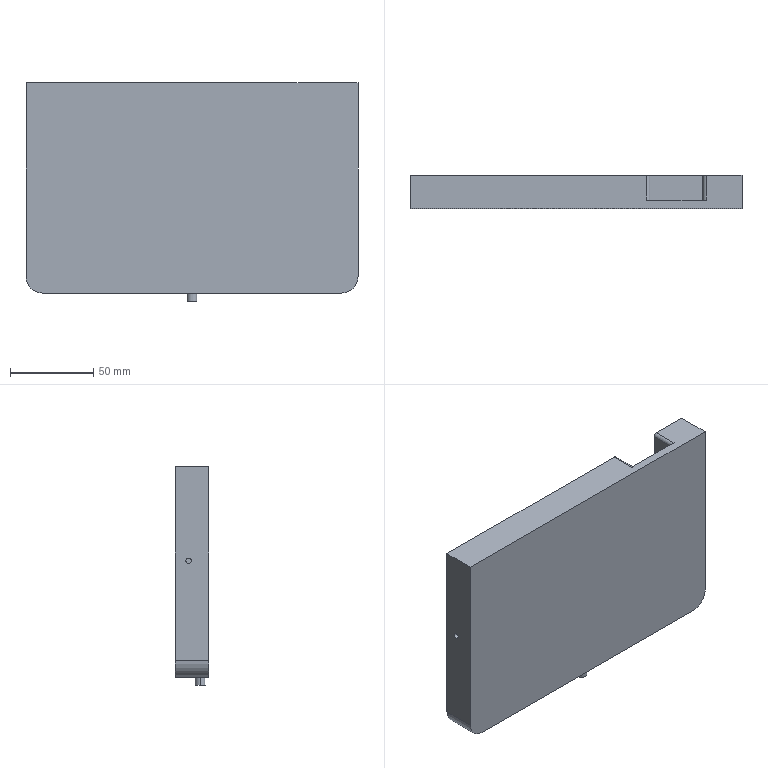Part | SolidWorks | features ICE 4, Fillet 3, HoleWzd 3, Extrusion 1 | 1 solid | 33 faces | box 200 x 20 x 131.788 mm | volume 297123 mm3 | cylinder 18 | plane 15 | commonest cylinder face diameters 4 x8 3.3 x4 5 x2 6 x2 20 x2
STEP:
#1=CARTESIAN_POINT('',(-58.35,12.,-50.));
#2=VERTEX_POINT('',#1);
#3=CARTESIAN_POINT('',(-61.65,12.,-50.));
#4=VERTEX_POINT('',#3);
#5=CARTESIAN_POINT('',(-60.,12.,-50.));
#6=DIRECTION('',(0.,0.,-1.));
#7=DIRECTION('',(-1.,0.,0.));
#8=AXIS2_PLACEMENT_3D('',#5,#6,#7);
#9=CIRCLE('',#8,1.65);
#10=EDGE_CURVE('',#2,#4,#9,.T.);
#11=ORIENTED_EDGE('',*,*,#10,.F.);
#12=CARTESIAN_POINT('',(-58.35,12.,-75.));
#13=VERTEX_POINT('',#12);
#14=CARTESIAN_POINT('',(-58.35,12.,-75.));
#15=DIRECTION('',(0.,0.,-1.));
#16=VECTOR('',#15,1000.);
#17=LINE('',#14,#16);
#18=EDGE_CURVE('',#2,#13,#17,.T.);
#19=ORIENTED_EDGE('',*,*,#18,.T.);
#20=CARTESIAN_POINT('',(-61.65,12.,-75.));
#21=VERTEX_POINT('',#20);
#22=CARTESIAN_POINT('',(-60.,12.,-75.));
#23=DIRECTION('',(0.,0.,-1.));
#24=DIRECTION('',(-1.,0.,0.));
#25=AXIS2_PLACEMENT_3D('',#22,#23,#24);
#26=CIRCLE('',#25,1.65);
#27=EDGE_CURVE('',#13,#21,#26,.T.);
#28=ORIENTED_EDGE('',*,*,#27,.T.);
#29=CARTESIAN_POINT('',(-61.65,12.,-75.));
#30=DIRECTION('',(0.,0.,-1.));
#31=VECTOR('',#30,1000.);
#32=LINE('',#29,#31);
#33=EDGE_CURVE('',#4,#21,#32,.T.);
#34=ORIENTED_EDGE('',*,*,#33,.F.);
#35=EDGE_LOOP('',(#11,#19,#28,#34));
#36=FACE_OUTER_BOUND('',#35,.T.);
#37=CARTESIAN_POINT('',(-60.,12.,-75.));
#38=DIRECTION('',(0.,0.,-1.));
#39=DIRECTION('',(-1.,0.,0.));
#40=AXIS2_PLACEMENT_3D('',#37,#38,#39);
#41=CYLINDRICAL_SURFACE('',#40,1.65);
#42=ADVANCED_FACE('',(#36),#41,.F.);
#43=CARTESIAN_POINT('',(-82.5,12.,-6.65));
#44=VERTEX_POINT('',#43);
#45=CARTESIAN_POINT('',(-82.5,12.,-3.35));
#46=VERTEX_POINT('',#45);
#47=CARTESIAN_POINT('',(-82.5,12.,-5.));
#48=DIRECTION('',(-1.,0.,0.));
#49=DIRECTION('',(0.,0.,1.));
#50=AXIS2_PLACEMENT_3D('',#47,#48,#49);
#51=CIRCLE('',#50,1.65);
#52=EDGE_CURVE('',#44,#46,#51,.T.);
#53=ORIENTED_EDGE('',*,*,#52,.F.);
#54=CARTESIAN_POINT('',(-100.,12.,-6.65));
#55=VERTEX_POINT('',#54);
#56=CARTESIAN_POINT('',(-100.,12.,-6.65));
#57=DIRECTION('',(-1.,0.,0.));
#58=VECTOR('',#57,1000.);
#59=LINE('',#56,#58);
#60=EDGE_CURVE('',#44,#55,#59,.T.);
#61=ORIENTED_EDGE('',*,*,#60,.T.);
#62=CARTESIAN_POINT('',(-100.,12.,-3.35));
#63=VERTEX_POINT('',#62);
#64=CARTESIAN_POINT('',(-100.,12.,-5.));
#65=DIRECTION('',(-1.,0.,0.));
#66=DIRECTION('',(0.,0.,1.));
#67=AXIS2_PLACEMENT_3D('',#64,#65,#66);
#68=CIRCLE('',#67,1.65);
#69=EDGE_CURVE('',#55,#63,#68,.T.);
#70=ORIENTED_EDGE('',*,*,#69,.T.);
#71=CARTESIAN_POINT('',(-100.,12.,-3.35));
#72=DIRECTION('',(-1.,0.,0.));
#73=VECTOR('',#72,1000.);
#74=LINE('',#71,#73);
#75=EDGE_CURVE('',#46,#63,#74,.T.);
#76=ORIENTED_EDGE('',*,*,#75,.F.);
#77=EDGE_LOOP('',(#53,#61,#70,#76));
#78=FACE_OUTER_BOUND('',#77,.T.);
#79=CARTESIAN_POINT('',(-100.,12.,-5.));
#80=DIRECTION('',(-1.,0.,0.));
#81=DIRECTION('',(0.,0.,1.));
#82=AXIS2_PLACEMENT_3D('',#79,#80,#81);
#83=CYLINDRICAL_SURFACE('',#82,1.65);
#84=ADVANCED_FACE('',(#78),#83,.F.);
#85=CARTESIAN_POINT('',(-2.5,14.,-50.));
#86=VERTEX_POINT('',#85);
#87=CARTESIAN_POINT('',(2.5,14.,-50.));
#88=VERTEX_POINT('',#87);
#89=CARTESIAN_POINT('',(0.,14.,-50.));
#90=DIRECTION('',(0.,0.,1.));
#91=DIRECTION('',(-1.,0.,0.));
#92=AXIS2_PLACEMENT_3D('',#89,#90,#91);
#93=CIRCLE('',#92,2.5);
#94=EDGE_CURVE('',#86,#88,#93,.T.);
#95=ORIENTED_EDGE('',*,*,#94,.T.);
#96=CARTESIAN_POINT('',(2.5,14.,-75.));
#97=VERTEX_POINT('',#96);
#98=CARTESIAN_POINT('',(2.5,14.,-75.));
#99=DIRECTION('',(0.,0.,-1.));
#100=VECTOR('',#99,1000.);
#101=LINE('',#98,#100);
#102=EDGE_CURVE('',#88,#97,#101,.T.);
#103=ORIENTED_EDGE('',*,*,#102,.T.);
#104=CARTESIAN_POINT('',(-2.5,14.,-75.));
#105=VERTEX_POINT('',#104);
#106=CARTESIAN_POINT('',(0.,14.,-75.));
#107=DIRECTION('',(0.,0.,-1.));
#108=DIRECTION('',(-1.,0.,0.));
#109=AXIS2_PLACEMENT_3D('',#106,#107,#108);
#110=CIRCLE('',#109,2.5);
#111=EDGE_CURVE('',#97,#105,#110,.T.);
#112=ORIENTED_EDGE('',*,*,#111,.T.);
#113=CARTESIAN_POINT('',(-2.5,14.,-75.));
#114=DIRECTION('',(0.,0.,-1.));
#115=VECTOR('',#114,1000.);
#116=LINE('',#113,#115);
#117=EDGE_CURVE('',#86,#105,#116,.T.);
#118=ORIENTED_EDGE('',*,*,#117,.F.);
#119=EDGE_LOOP('',(#95,#103,#112,#118));
#120=FACE_OUTER_BOUND('',#119,.T.);
#121=CARTESIAN_POINT('',(0.,14.,-75.));
#122=DIRECTION('',(0.,0.,-1.));
#123=DIRECTION('',(-1.,0.,0.));
#124=AXIS2_PLACEMENT_3D('',#121,#122,#123);
#125=CYLINDRICAL_SURFACE('',#124,2.5);
#126=ADVANCED_FACE('',(#120),#125,.F.);
#127=CARTESIAN_POINT('',(-3.,5.,-80.));
#128=VERTEX_POINT('',#127);
#129=CARTESIAN_POINT('',(3.,5.,-80.));
#130=VERTEX_POINT('',#129);
#131=CARTESIAN_POINT('',(0.,5.,-80.));
#132=DIRECTION('',(0.,0.,-1.));
#133=DIRECTION('',(-1.,0.,0.));
#134=AXIS2_PLACEMENT_3D('',#131,#132,#133);
#135=CIRCLE('',#134,3.);
#136=EDGE_CURVE('',#128,#130,#135,.T.);
#137=ORIENTED_EDGE('',*,*,#136,.F.);
#138=CARTESIAN_POINT('',(-3.,5.,-75.));
#139=VERTEX_POINT('',#138);
#140=CARTESIAN_POINT('',(-3.,5.,-80.));
#141=DIRECTION('',(0.,0.,1.));
#142=VECTOR('',#141,1000.);
#143=LINE('',#140,#142);
#144=EDGE_CURVE('',#128,#139,#143,.T.);
#145=ORIENTED_EDGE('',*,*,#144,.T.);
#146=CARTESIAN_POINT('',(3.,5.,-75.));
#147=VERTEX_POINT('',#146);
#148=CARTESIAN_POINT('',(0.,5.,-75.));
#149=DIRECTION('',(0.,0.,-1.));
#150=DIRECTION('',(1.,0.,0.));
#151=AXIS2_PLACEMENT_3D('',#148,#149,#150);
#152=CIRCLE('',#151,3.);
#153=EDGE_CURVE('',#139,#147,#152,.T.);
#154=ORIENTED_EDGE('',*,*,#153,.T.);
#155=CARTESIAN_POINT('',(3.,5.,-80.));
#156=DIRECTION('',(0.,0.,1.));
#157=VECTOR('',#156,1000.);
#158=LINE('',#155,#157);
#159=EDGE_CURVE('',#130,#147,#158,.T.);
#160=ORIENTED_EDGE('',*,*,#159,.F.);
#161=EDGE_LOOP('',(#137,#145,#154,#160));
#162=FACE_OUTER_BOUND('',#161,.T.);
#163=CARTESIAN_POINT('',(0.,5.,-80.));
#164=DIRECTION('',(0.,0.,1.));
#165=DIRECTION('',(1.,0.,0.));
#166=AXIS2_PLACEMENT_3D('',#163,#164,#165);
#167=CYLINDRICAL_SURFACE('',#166,3.);
#168=ADVANCED_FACE('',(#162),#167,.T.);
#169=CARTESIAN_POINT('',(100.,20.,51.788));
#170=VERTEX_POINT('',#169);
#171=CARTESIAN_POINT('',(100.,20.,-65.));
#172=VERTEX_POINT('',#171);
#173=CARTESIAN_POINT('',(100.,20.,75.));
#174=DIRECTION('',(0.,0.,-1.));
#175=VECTOR('',#174,1000.);
#176=LINE('',#173,#175);
#177=EDGE_CURVE('',#170,#172,#176,.T.);
#178=ORIENTED_EDGE('',*,*,#177,.F.);
#179=CARTESIAN_POINT('',(100.,0.,51.788));
#180=VERTEX_POINT('',#179);
#181=CARTESIAN_POINT('',(100.,20.,51.788));
#182=DIRECTION('',(0.,-1.,0.));
#183=VECTOR('',#182,1000.);
#184=LINE('',#181,#183);
#185=EDGE_CURVE('',#170,#180,#184,.T.);
#186=ORIENTED_EDGE('',*,*,#185,.T.);
#187=CARTESIAN_POINT('',(100.,0.,-65.));
#188=VERTEX_POINT('',#187);
#189=CARTESIAN_POINT('',(100.,0.,75.));
#190=DIRECTION('',(0.,0.,-1.));
#191=VECTOR('',#190,1000.);
#192=LINE('',#189,#191);
#193=EDGE_CURVE('',#180,#188,#192,.T.);
#194=ORIENTED_EDGE('',*,*,#193,.T.);
#195=CARTESIAN_POINT('',(100.,20.,-65.));
#196=DIRECTION('',(0.,1.,0.));
#197=VECTOR('',#196,1000.);
#198=LINE('',#195,#197);
#199=EDGE_CURVE('',#188,#172,#198,.T.);
#200=ORIENTED_EDGE('',*,*,#199,.T.);
#201=EDGE_LOOP('',(#178,#186,#194,#200));
#202=FACE_OUTER_BOUND('',#201,.T.);
#203=CARTESIAN_POINT('',(100.,20.,75.));
#204=DIRECTION('',(-1.,0.,0.));
#205=DIRECTION('',(0.,0.,1.));
#206=AXIS2_PLACEMENT_3D('',#203,#204,#205);
#207=PLANE('',#206);
#208=ADVANCED_FACE('',(#202),#207,.F.);
#209=CARTESIAN_POINT('',(-60.,12.,-75.));
#210=DIRECTION('',(0.,0.,-1.));
#211=DIRECTION('',(-1.,0.,0.));
#212=AXIS2_PLACEMENT_3D('',#209,#210,#211);
#213=CIRCLE('',#212,1.65);
#214=EDGE_CURVE('',#21,#13,#213,.T.);
#215=ORIENTED_EDGE('',*,*,#214,.F.);
#216=ORIENTED_EDGE('',*,*,#27,.F.);
#217=EDGE_LOOP('',(#215,#216));
#218=FACE_BOUND('',#217,.T.);
#219=CARTESIAN_POINT('',(0.,14.,-75.));
#220=DIRECTION('',(0.,0.,-1.));
#221=DIRECTION('',(-1.,0.,0.));
#222=AXIS2_PLACEMENT_3D('',#219,#220,#221);
#223=CIRCLE('',#222,2.5);
#224=EDGE_CURVE('',#105,#97,#223,.T.);
#225=ORIENTED_EDGE('',*,*,#224,.F.);
#226=ORIENTED_EDGE('',*,*,#111,.F.);
#227=EDGE_LOOP('',(#225,#226));
#228=FACE_BOUND('',#227,.T.);
#229=CARTESIAN_POINT('',(0.,5.,-75.));
#230=DIRECTION('',(0.,0.,-1.));
#231=DIRECTION('',(1.,0.,0.));
#232=AXIS2_PLACEMENT_3D('',#229,#230,#231);
#233=CIRCLE('',#232,3.);
#234=EDGE_CURVE('',#147,#139,#233,.T.);
#235=ORIENTED_EDGE('',*,*,#234,.F.);
#236=ORIENTED_EDGE('',*,*,#153,.F.);
#237=EDGE_LOOP('',(#235,#236));
#238=FACE_BOUND('',#237,.T.);
#239=CARTESIAN_POINT('',(90.,20.,-75.));
#240=VERTEX_POINT('',#239);
#241=CARTESIAN_POINT('',(-90.,20.,-75.));
#242=VERTEX_POINT('',#241);
#243=CARTESIAN_POINT('',(-100.,20.,-75.));
#244=DIRECTION('',(-1.,0.,0.));
#245=VECTOR('',#244,1000.);
#246=LINE('',#243,#245);
#247=EDGE_CURVE('',#240,#242,#246,.T.);
#248=ORIENTED_EDGE('',*,*,#247,.F.);
#249=CARTESIAN_POINT('',(90.,0.,-75.));
#250=VERTEX_POINT('',#249);
#251=CARTESIAN_POINT('',(90.,20.,-75.));
#252=DIRECTION('',(0.,-1.,0.));
#253=VECTOR('',#252,1000.);
#254=LINE('',#251,#253);
#255=EDGE_CURVE('',#240,#250,#254,.T.);
#256=ORIENTED_EDGE('',*,*,#255,.T.);
#257=CARTESIAN_POINT('',(-90.,0.,-75.));
#258=VERTEX_POINT('',#257);
#259=CARTESIAN_POINT('',(-100.,0.,-75.));
#260=DIRECTION('',(-1.,0.,0.));
#261=VECTOR('',#260,1000.);
#262=LINE('',#259,#261);
#263=EDGE_CURVE('',#250,#258,#262,.T.);
#264=ORIENTED_EDGE('',*,*,#263,.T.);
#265=CARTESIAN_POINT('',(-90.,20.,-75.));
#266=DIRECTION('',(0.,1.,0.));
#267=VECTOR('',#266,1000.);
#268=LINE('',#265,#267);
#269=EDGE_CURVE('',#258,#242,#268,.T.);
#270=ORIENTED_EDGE('',*,*,#269,.T.);
#271=EDGE_LOOP('',(#248,#256,#264,#270));
#272=FACE_OUTER_BOUND('',#271,.T.);
#273=CARTESIAN_POINT('',(-100.,20.,-75.));
#274=DIRECTION('',(0.,0.,1.));
#275=DIRECTION('',(1.,0.,0.));
#276=AXIS2_PLACEMENT_3D('',#273,#274,#275);
#277=PLANE('',#276);
#278=ADVANCED_FACE('',(#218,#228,#238,#272),#277,.F.);
#279=CARTESIAN_POINT('',(-100.,12.,-5.));
#280=DIRECTION('',(-1.,0.,0.));
#281=DIRECTION('',(0.,0.,1.));
#282=AXIS2_PLACEMENT_3D('',#279,#280,#281);
#283=CIRCLE('',#282,1.65);
#284=EDGE_CURVE('',#63,#55,#283,.T.);
#285=ORIENTED_EDGE('',*,*,#284,.F.);
#286=ORIENTED_EDGE('',*,*,#69,.F.);
#287=EDGE_LOOP('',(#285,#286));
#288=FACE_BOUND('',#287,.T.);
#289=CARTESIAN_POINT('',(-100.,0.,-65.));
#290=VERTEX_POINT('',#289);
#291=CARTESIAN_POINT('',(-100.,0.,51.788));
#292=VERTEX_POINT('',#291);
#293=CARTESIAN_POINT('',(-100.,0.,75.));
#294=DIRECTION('',(0.,0.,1.));
#295=VECTOR('',#294,1000.);
#296=LINE('',#293,#295);
#297=EDGE_CURVE('',#290,#292,#296,.T.);
#298=ORIENTED_EDGE('',*,*,#297,.T.);
#299=CARTESIAN_POINT('',(-100.,20.,51.788));
#300=VERTEX_POINT('',#299);
#301=CARTESIAN_POINT('',(-100.,20.,51.788));
#302=DIRECTION('',(0.,1.,0.));
#303=VECTOR('',#302,1000.);
#304=LINE('',#301,#303);
#305=EDGE_CURVE('',#292,#300,#304,.T.);
#306=ORIENTED_EDGE('',*,*,#305,.T.);
#307=CARTESIAN_POINT('',(-100.,20.,-65.));
#308=VERTEX_POINT('',#307);
#309=CARTESIAN_POINT('',(-100.,20.,75.));
#310=DIRECTION('',(0.,0.,1.));
#311=VECTOR('',#310,1000.);
#312=LINE('',#309,#311);
#313=EDGE_CURVE('',#308,#300,#312,.T.);
#314=ORIENTED_EDGE('',*,*,#313,.F.);
#315=CARTESIAN_POINT('',(-100.,20.,-65.));
#316=DIRECTION('',(0.,-1.,0.));
#317=VECTOR('',#316,1000.);
#318=LINE('',#315,#317);
#319=EDGE_CURVE('',#308,#290,#318,.T.);
#320=ORIENTED_EDGE('',*,*,#319,.T.);
#321=EDGE_LOOP('',(#298,#306,#314,#320));
#322=FACE_OUTER_BOUND('',#321,.T.);
#323=CARTESIAN_POINT('',(-100.,20.,75.));
#324=DIRECTION('',(1.,0.,0.));
#325=DIRECTION('',(0.,0.,-1.));
#326=AXIS2_PLACEMENT_3D('',#323,#324,#325);
#327=PLANE('',#326);
#328=ADVANCED_FACE('',(#288,#322),#327,.F.);
#329=CARTESIAN_POINT('',(42.5,20.,51.788));
#330=VERTEX_POINT('',#329);
#331=CARTESIAN_POINT('',(73.5,20.,51.788));
#332=DIRECTION('',(-1.,0.,0.));
#333=VECTOR('',#332,1000.);
#334=LINE('',#331,#333);
#335=EDGE_CURVE('',#330,#300,#334,.T.);
#336=ORIENTED_EDGE('',*,*,#335,.F.);
#337=CARTESIAN_POINT('',(44.5,20.,49.788));
#338=VERTEX_POINT('',#337);
#339=CARTESIAN_POINT('',(42.5,20.,49.788));
#340=DIRECTION('',(0.,1.,0.));
#341=DIRECTION('',(0.,0.,-1.));
#342=AXIS2_PLACEMENT_3D('',#339,#340,#341);
#343=CIRCLE('',#342,2.);
#344=EDGE_CURVE('',#330,#338,#343,.T.);
#345=ORIENTED_EDGE('',*,*,#344,.T.);
#346=CARTESIAN_POINT('',(44.5,20.,32.));
#347=VERTEX_POINT('',#346);
#348=CARTESIAN_POINT('',(44.5,20.,30.));
#349=DIRECTION('',(0.,0.,1.));
#350=VECTOR('',#349,1000.);
#351=LINE('',#348,#350);
#352=EDGE_CURVE('',#347,#338,#351,.T.);
#353=ORIENTED_EDGE('',*,*,#352,.F.);
#354=CARTESIAN_POINT('',(42.5,20.,30.));
#355=VERTEX_POINT('',#354);
#356=CARTESIAN_POINT('',(42.5,20.,32.));
#357=DIRECTION('',(0.,1.,0.));
#358=DIRECTION('',(0.,0.,-1.));
#359=AXIS2_PLACEMENT_3D('',#356,#357,#358);
#360=CIRCLE('',#359,2.);
#361=EDGE_CURVE('',#347,#355,#360,.T.);
#362=ORIENTED_EDGE('',*,*,#361,.T.);
#363=CARTESIAN_POINT('',(-80.5,20.,30.));
#364=VERTEX_POINT('',#363);
#365=CARTESIAN_POINT('',(-82.5,20.,30.));
#366=DIRECTION('',(1.,0.,0.));
#367=VECTOR('',#366,1000.);
#368=LINE('',#365,#367);
#369=EDGE_CURVE('',#364,#355,#368,.T.);
#370=ORIENTED_EDGE('',*,*,#369,.F.);
#371=CARTESIAN_POINT('',(-82.5,20.,28.));
#372=VERTEX_POINT('',#371);
#373=CARTESIAN_POINT('',(-80.5,20.,28.));
#374=DIRECTION('',(0.,-1.,0.));
#375=DIRECTION('',(0.,0.,-1.));
#376=AXIS2_PLACEMENT_3D('',#373,#374,#375);
#377=CIRCLE('',#376,2.);
#378=EDGE_CURVE('',#364,#372,#377,.T.);
#379=ORIENTED_EDGE('',*,*,#378,.T.);
#380=CARTESIAN_POINT('',(-82.5,20.,-48.));
#381=VERTEX_POINT('',#380);
#382=CARTESIAN_POINT('',(-82.5,20.,-50.));
#383=DIRECTION('',(0.,0.,1.));
#384=VECTOR('',#383,1000.);
#385=LINE('',#382,#384);
#386=EDGE_CURVE('',#381,#372,#385,.T.);
#387=ORIENTED_EDGE('',*,*,#386,.F.);
#388=CARTESIAN_POINT('',(-80.5,20.,-50.));
#389=VERTEX_POINT('',#388);
#390=CARTESIAN_POINT('',(-80.5,20.,-48.));
#391=DIRECTION('',(0.,-1.,0.));
#392=DIRECTION('',(0.,0.,-1.));
#393=AXIS2_PLACEMENT_3D('',#390,#391,#392);
#394=CIRCLE('',#393,2.);
#395=EDGE_CURVE('',#381,#389,#394,.T.);
#396=ORIENTED_EDGE('',*,*,#395,.T.);
#397=CARTESIAN_POINT('',(80.5,20.,-50.));
#398=VERTEX_POINT('',#397);
#399=CARTESIAN_POINT('',(-82.5,20.,-50.));
#400=DIRECTION('',(-1.,0.,0.));
#401=VECTOR('',#400,1000.);
#402=LINE('',#399,#401);
#403=EDGE_CURVE('',#398,#389,#402,.T.);
#404=ORIENTED_EDGE('',*,*,#403,.F.);
#405=CARTESIAN_POINT('',(82.5,20.,-48.));
#406=VERTEX_POINT('',#405);
#407=CARTESIAN_POINT('',(80.5,20.,-48.));
#408=DIRECTION('',(0.,-1.,0.));
#409=DIRECTION('',(0.,0.,-1.));
#410=AXIS2_PLACEMENT_3D('',#407,#408,#409);
#411=CIRCLE('',#410,2.);
#412=EDGE_CURVE('',#398,#406,#411,.T.);
#413=ORIENTED_EDGE('',*,*,#412,.T.);
#414=CARTESIAN_POINT('',(82.5,20.,28.));
#415=VERTEX_POINT('',#414);
#416=CARTESIAN_POINT('',(82.5,20.,-50.));
#417=DIRECTION('',(0.,0.,-1.));
#418=VECTOR('',#417,1000.);
#419=LINE('',#416,#418);
#420=EDGE_CURVE('',#415,#406,#419,.T.);
#421=ORIENTED_EDGE('',*,*,#420,.F.);
#422=CARTESIAN_POINT('',(80.5,20.,30.));
#423=VERTEX_POINT('',#422);
#424=CARTESIAN_POINT('',(80.5,20.,28.));
#425=DIRECTION('',(0.,-1.,0.));
#426=DIRECTION('',(0.,0.,-1.));
#427=AXIS2_PLACEMENT_3D('',#424,#425,#426);
#428=CIRCLE('',#427,2.);
#429=EDGE_CURVE('',#415,#423,#428,.T.);
#430=ORIENTED_EDGE('',*,*,#429,.T.);
#431=CARTESIAN_POINT('',(78.5,20.,30.));
#432=VERTEX_POINT('',#431);
#433=CARTESIAN_POINT('',(82.5,20.,30.));
#434=DIRECTION('',(1.,0.,0.));
#435=VECTOR('',#434,1000.);
#436=LINE('',#433,#435);
#437=EDGE_CURVE('',#432,#423,#436,.T.);
#438=ORIENTED_EDGE('',*,*,#437,.F.);
#439=CARTESIAN_POINT('',(76.5,20.,32.));
#440=VERTEX_POINT('',#439);
#441=CARTESIAN_POINT('',(78.5,20.,32.));
#442=DIRECTION('',(0.,1.,0.));
#443=DIRECTION('',(0.,0.,-1.));
#444=AXIS2_PLACEMENT_3D('',#441,#442,#443);
#445=CIRCLE('',#444,2.);
#446=EDGE_CURVE('',#432,#440,#445,.T.);
#447=ORIENTED_EDGE('',*,*,#446,.T.);
#448=CARTESIAN_POINT('',(76.5,20.,49.788));
#449=VERTEX_POINT('',#448);
#450=CARTESIAN_POINT('',(76.5,20.,51.788));
#451=DIRECTION('',(0.,0.,-1.));
#452=VECTOR('',#451,1000.);
#453=LINE('',#450,#452);
#454=EDGE_CURVE('',#449,#440,#453,.T.);
#455=ORIENTED_EDGE('',*,*,#454,.F.);
#456=CARTESIAN_POINT('',(78.5,20.,51.788));
#457=VERTEX_POINT('',#456);
#458=CARTESIAN_POINT('',(78.5,20.,49.788));
#459=DIRECTION('',(0.,1.,0.));
#460=DIRECTION('',(0.,0.,-1.));
#461=AXIS2_PLACEMENT_3D('',#458,#459,#460);
#462=CIRCLE('',#461,2.);
#463=EDGE_CURVE('',#449,#457,#462,.T.);
#464=ORIENTED_EDGE('',*,*,#463,.T.);
#465=CARTESIAN_POINT('',(73.5,20.,51.788));
#466=DIRECTION('',(-1.,0.,0.));
#467=VECTOR('',#466,1000.);
#468=LINE('',#465,#467);
#469=EDGE_CURVE('',#170,#457,#468,.T.);
#470=ORIENTED_EDGE('',*,*,#469,.F.);
#471=ORIENTED_EDGE('',*,*,#177,.T.);
#472=CARTESIAN_POINT('',(90.,20.,-65.));
#473=DIRECTION('',(0.,1.,0.));
#474=DIRECTION('',(0.,0.,-1.));
#475=AXIS2_PLACEMENT_3D('',#472,#473,#474);
#476=CIRCLE('',#475,10.);
#477=EDGE_CURVE('',#172,#240,#476,.T.);
#478=ORIENTED_EDGE('',*,*,#477,.T.);
#479=ORIENTED_EDGE('',*,*,#247,.T.);
#480=CARTESIAN_POINT('',(-90.,20.,-65.));
#481=DIRECTION('',(0.,1.,0.));
#482=DIRECTION('',(0.,0.,-1.));
#483=AXIS2_PLACEMENT_3D('',#480,#481,#482);
#484=CIRCLE('',#483,10.);
#485=EDGE_CURVE('',#242,#308,#484,.T.);
#486=ORIENTED_EDGE('',*,*,#485,.T.);
#487=ORIENTED_EDGE('',*,*,#313,.T.);
#488=EDGE_LOOP('',(#336,#345,#353,#362,#370,#379,#387,#396,#404,#413,#421,#430,#438,#447,#455,#464,#470,#471,#478,#479,#486,#487));
#489=FACE_OUTER_BOUND('',#488,.T.);
#490=CARTESIAN_POINT('',(0.,20.,0.));
#491=DIRECTION('',(0.,-1.,0.));
#492=DIRECTION('',(0.,0.,-1.));
#493=AXIS2_PLACEMENT_3D('',#490,#491,#492);
#494=PLANE('',#493);
#495=ADVANCED_FACE('',(#489),#494,.F.);
#496=CARTESIAN_POINT('',(68.5,0.,51.788));
#497=DIRECTION('',(-1.,0.,0.));
#498=VECTOR('',#497,1000.);
#499=LINE('',#496,#498);
#500=EDGE_CURVE('',#180,#292,#499,.T.);
#501=ORIENTED_EDGE('',*,*,#500,.T.);
#502=ORIENTED_EDGE('',*,*,#297,.F.);
#503=CARTESIAN_POINT('',(-90.,0.,-65.));
#504=DIRECTION('',(0.,-1.,0.));
#505=DIRECTION('',(0.,0.,-1.));
#506=AXIS2_PLACEMENT_3D('',#503,#504,#505);
#507=CIRCLE('',#506,10.);
#508=EDGE_CURVE('',#290,#258,#507,.T.);
#509=ORIENTED_EDGE('',*,*,#508,.T.);
#510=ORIENTED_EDGE('',*,*,#263,.F.);
#511=CARTESIAN_POINT('',(90.,0.,-65.));
#512=DIRECTION('',(0.,-1.,0.));
#513=DIRECTION('',(0.,0.,-1.));
#514=AXIS2_PLACEMENT_3D('',#511,#512,#513);
#515=CIRCLE('',#514,10.);
#516=EDGE_CURVE('',#250,#188,#515,.T.);
#517=ORIENTED_EDGE('',*,*,#516,.T.);
#518=ORIENTED_EDGE('',*,*,#193,.F.);
#519=EDGE_LOOP('',(#501,#502,#509,#510,#517,#518));
#520=FACE_OUTER_BOUND('',#519,.T.);
#521=CARTESIAN_POINT('',(0.,0.,0.));
#522=DIRECTION('',(0.,-1.,0.));
#523=DIRECTION('',(0.,0.,-1.));
#524=AXIS2_PLACEMENT_3D('',#521,#522,#523);
#525=PLANE('',#524);
#526=ADVANCED_FACE('',(#520),#525,.T.);
#527=ORIENTED_EDGE('',*,*,#144,.F.);
#528=CARTESIAN_POINT('',(0.,5.,-80.));
#529=DIRECTION('',(0.,0.,-1.));
#530=DIRECTION('',(-1.,0.,0.));
#531=AXIS2_PLACEMENT_3D('',#528,#529,#530);
#532=CIRCLE('',#531,3.);
#533=EDGE_CURVE('',#130,#128,#532,.T.);
#534=ORIENTED_EDGE('',*,*,#533,.F.);
#535=ORIENTED_EDGE('',*,*,#159,.T.);
#536=ORIENTED_EDGE('',*,*,#234,.T.);
#537=EDGE_LOOP('',(#527,#534,#535,#536));
#538=FACE_OUTER_BOUND('',#537,.T.);
#539=CARTESIAN_POINT('',(0.,5.,-80.));
#540=DIRECTION('',(0.,0.,1.));
#541=DIRECTION('',(1.,0.,0.));
#542=AXIS2_PLACEMENT_3D('',#539,#540,#541);
#543=CYLINDRICAL_SURFACE('',#542,3.);
#544=ADVANCED_FACE('',(#538),#543,.T.);
#545=ORIENTED_EDGE('',*,*,#533,.T.);
#546=ORIENTED_EDGE('',*,*,#136,.T.);
#547=EDGE_LOOP('',(#545,#546));
#548=FACE_OUTER_BOUND('',#547,.T.);
#549=CARTESIAN_POINT('',(0.,5.,-80.));
#550=DIRECTION('',(0.,0.,-1.));
#551=DIRECTION('',(-1.,0.,0.));
#552=AXIS2_PLACEMENT_3D('',#549,#550,#551);
#553=PLANE('',#552);
#554=ADVANCED_FACE('',(#548),#553,.T.);
#555=ORIENTED_EDGE('',*,*,#102,.F.);
#556=CARTESIAN_POINT('',(0.,14.,-50.));
#557=DIRECTION('',(0.,0.,1.));
#558=DIRECTION('',(-1.,0.,0.));
#559=AXIS2_PLACEMENT_3D('',#556,#557,#558);
#560=CIRCLE('',#559,2.5);
#561=EDGE_CURVE('',#88,#86,#560,.T.);
#562=ORIENTED_EDGE('',*,*,#561,.T.);
#563=ORIENTED_EDGE('',*,*,#117,.T.);
#564=ORIENTED_EDGE('',*,*,#224,.T.);
#565=EDGE_LOOP('',(#555,#562,#563,#564));
#566=FACE_OUTER_BOUND('',#565,.T.);
#567=CARTESIAN_POINT('',(0.,14.,-75.));
#568=DIRECTION('',(0.,0.,-1.));
#569=DIRECTION('',(-1.,0.,0.));
#570=AXIS2_PLACEMENT_3D('',#567,#568,#569);
#571=CYLINDRICAL_SURFACE('',#570,2.5);
#572=ADVANCED_FACE('',(#566),#571,.F.);
#573=CARTESIAN_POINT('',(-60.,12.,-50.));
#574=DIRECTION('',(0.,0.,-1.));
#575=DIRECTION('',(-1.,0.,0.));
#576=AXIS2_PLACEMENT_3D('',#573,#574,#575);
#577=CIRCLE('',#576,1.65);
#578=EDGE_CURVE('',#4,#2,#577,.T.);
#579=ORIENTED_EDGE('',*,*,#578,.T.);
#580=ORIENTED_EDGE('',*,*,#10,.T.);
#581=EDGE_LOOP('',(#579,#580));
#582=FACE_BOUND('',#581,.T.);
#583=ORIENTED_EDGE('',*,*,#403,.T.);
#584=CARTESIAN_POINT('',(-80.5,5.,-50.));
#585=VERTEX_POINT('',#584);
#586=CARTESIAN_POINT('',(-80.5,5.,-50.));
#587=DIRECTION('',(0.,-1.,0.));
#588=VECTOR('',#587,1000.);
#589=LINE('',#586,#588);
#590=EDGE_CURVE('',#389,#585,#589,.T.);
#591=ORIENTED_EDGE('',*,*,#590,.T.);
#592=CARTESIAN_POINT('',(80.5,5.,-50.));
#593=VERTEX_POINT('',#592);
#594=CARTESIAN_POINT('',(76.5,5.,-50.));
#595=DIRECTION('',(-1.,0.,0.));
#596=VECTOR('',#595,1000.);
#597=LINE('',#594,#596);
#598=EDGE_CURVE('',#593,#585,#597,.T.);
#599=ORIENTED_EDGE('',*,*,#598,.F.);
#600=CARTESIAN_POINT('',(80.5,20.,-50.));
#601=DIRECTION('',(0.,1.,0.));
#602=VECTOR('',#601,1000.);
#603=LINE('',#600,#602);
#604=EDGE_CURVE('',#593,#398,#603,.T.);
#605=ORIENTED_EDGE('',*,*,#604,.T.);
#606=EDGE_LOOP('',(#583,#591,#599,#605));
#607=FACE_OUTER_BOUND('',#606,.T.);
#608=ORIENTED_EDGE('',*,*,#94,.F.);
#609=ORIENTED_EDGE('',*,*,#561,.F.);
#610=EDGE_LOOP('',(#608,#609));
#611=FACE_BOUND('',#610,.T.);
#612=CARTESIAN_POINT('',(-82.5,5.,-50.));
#613=DIRECTION('',(0.,0.,-1.));
#614=DIRECTION('',(-1.,0.,0.));
#615=AXIS2_PLACEMENT_3D('',#612,#613,#614);
#616=PLANE('',#615);
#617=ADVANCED_FACE('',(#582,#607,#611),#616,.F.);
#618=CARTESIAN_POINT('',(-82.5,12.,-5.));
#619=DIRECTION('',(-1.,0.,0.));
#620=DIRECTION('',(0.,0.,1.));
#621=AXIS2_PLACEMENT_3D('',#618,#619,#620);
#622=CIRCLE('',#621,1.65);
#623=EDGE_CURVE('',#46,#44,#622,.T.);
#624=ORIENTED_EDGE('',*,*,#623,.T.);
#625=ORIENTED_EDGE('',*,*,#52,.T.);
#626=EDGE_LOOP('',(#624,#625));
#627=FACE_BOUND('',#626,.T.);
#628=CARTESIAN_POINT('',(-82.5,5.,-48.));
#629=VERTEX_POINT('',#628);
#630=CARTESIAN_POINT('',(-82.5,5.,28.));
#631=VERTEX_POINT('',#630);
#632=CARTESIAN_POINT('',(-82.5,5.,-50.));
#633=DIRECTION('',(0.,0.,1.));
#634=VECTOR('',#633,1000.);
#635=LINE('',#632,#634);
#636=EDGE_CURVE('',#629,#631,#635,.T.);
#637=ORIENTED_EDGE('',*,*,#636,.F.);
#638=CARTESIAN_POINT('',(-82.5,20.,-48.));
#639=DIRECTION('',(0.,1.,0.));
#640=VECTOR('',#639,1000.);
#641=LINE('',#638,#640);
#642=EDGE_CURVE('',#629,#381,#641,.T.);
#643=ORIENTED_EDGE('',*,*,#642,.T.);
#644=ORIENTED_EDGE('',*,*,#386,.T.);
#645=CARTESIAN_POINT('',(-82.5,5.,28.));
#646=DIRECTION('',(0.,-1.,0.));
#647=VECTOR('',#646,1000.);
#648=LINE('',#645,#647);
#649=EDGE_CURVE('',#372,#631,#648,.T.);
#650=ORIENTED_EDGE('',*,*,#649,.T.);
#651=EDGE_LOOP('',(#637,#643,#644,#650));
#652=FACE_OUTER_BOUND('',#651,.T.);
#653=CARTESIAN_POINT('',(-82.5,5.,-50.));
#654=DIRECTION('',(-1.,0.,0.));
#655=DIRECTION('',(0.,0.,1.));
#656=AXIS2_PLACEMENT_3D('',#653,#654,#655);
#657=PLANE('',#656);
#658=ADVANCED_FACE('',(#627,#652),#657,.F.);
#659=CARTESIAN_POINT('',(82.5,5.,28.));
#660=VERTEX_POINT('',#659);
#661=CARTESIAN_POINT('',(82.5,5.,-48.));
#662=VERTEX_POINT('',#661);
#663=CARTESIAN_POINT('',(82.5,5.,-50.));
#664=DIRECTION('',(0.,0.,-1.));
#665=VECTOR('',#664,1000.);
#666=LINE('',#663,#665);
#667=EDGE_CURVE('',#660,#662,#666,.T.);
#668=ORIENTED_EDGE('',*,*,#667,.F.);
#669=CARTESIAN_POINT('',(82.5,20.,28.));
#670=DIRECTION('',(0.,1.,0.));
#671=VECTOR('',#670,1000.);
#672=LINE('',#669,#671);
#673=EDGE_CURVE('',#660,#415,#672,.T.);
#674=ORIENTED_EDGE('',*,*,#673,.T.);
#675=ORIENTED_EDGE('',*,*,#420,.T.);
#676=CARTESIAN_POINT('',(82.5,5.,-48.));
#677=DIRECTION('',(0.,-1.,0.));
#678=VECTOR('',#677,1000.);
#679=LINE('',#676,#678);
#680=EDGE_CURVE('',#406,#662,#679,.T.);
#681=ORIENTED_EDGE('',*,*,#680,.T.);
#682=EDGE_LOOP('',(#668,#674,#675,#681));
#683=FACE_OUTER_BOUND('',#682,.T.);
#684=CARTESIAN_POINT('',(82.5,5.,-50.));
#685=DIRECTION('',(1.,0.,0.));
#686=DIRECTION('',(0.,0.,-1.));
#687=AXIS2_PLACEMENT_3D('',#684,#685,#686);
#688=PLANE('',#687);
#689=ADVANCED_FACE('',(#683),#688,.F.);
#690=CARTESIAN_POINT('',(78.5,5.,30.));
#691=VERTEX_POINT('',#690);
#692=CARTESIAN_POINT('',(80.5,5.,30.));
#693=VERTEX_POINT('',#692);
#694=CARTESIAN_POINT('',(82.5,5.,30.));
#695=DIRECTION('',(1.,0.,0.));
#696=VECTOR('',#695,1000.);
#697=LINE('',#694,#696);
#698=EDGE_CURVE('',#691,#693,#697,.T.);
#699=ORIENTED_EDGE('',*,*,#698,.F.);
#700=CARTESIAN_POINT('',(78.5,5.,30.));
#701=DIRECTION('',(0.,1.,0.));
#702=VECTOR('',#701,1000.);
#703=LINE('',#700,#702);
#704=EDGE_CURVE('',#691,#432,#703,.T.);
#705=ORIENTED_EDGE('',*,*,#704,.T.);
#706=ORIENTED_EDGE('',*,*,#437,.T.);
#707=CARTESIAN_POINT('',(80.5,5.,30.));
#708=DIRECTION('',(0.,-1.,0.));
#709=VECTOR('',#708,1000.);
#710=LINE('',#707,#709);
#711=EDGE_CURVE('',#423,#693,#710,.T.);
#712=ORIENTED_EDGE('',*,*,#711,.T.);
#713=EDGE_LOOP('',(#699,#705,#706,#712));
#714=FACE_OUTER_BOUND('',#713,.T.);
#715=CARTESIAN_POINT('',(82.5,5.,30.));
#716=DIRECTION('',(0.,0.,1.));
#717=DIRECTION('',(1.,0.,0.));
#718=AXIS2_PLACEMENT_3D('',#715,#716,#717);
#719=PLANE('',#718);
#720=ADVANCED_FACE('',(#714),#719,.F.);
#721=CARTESIAN_POINT('',(76.5,5.,49.788));
#722=VERTEX_POINT('',#721);
#723=CARTESIAN_POINT('',(76.5,5.,32.));
#724=VERTEX_POINT('',#723);
#725=CARTESIAN_POINT('',(76.5,5.,51.788));
#726=DIRECTION('',(0.,0.,-1.));
#727=VECTOR('',#726,1000.);
#728=LINE('',#725,#727);
#729=EDGE_CURVE('',#722,#724,#728,.T.);
#730=ORIENTED_EDGE('',*,*,#729,.F.);
#731=CARTESIAN_POINT('',(76.5,5.,49.788));
#732=DIRECTION('',(0.,1.,0.));
#733=VECTOR('',#732,1000.);
#734=LINE('',#731,#733);
#735=EDGE_CURVE('',#722,#449,#734,.T.);
#736=ORIENTED_EDGE('',*,*,#735,.T.);
#737=ORIENTED_EDGE('',*,*,#454,.T.);
#738=CARTESIAN_POINT('',(76.5,5.,32.));
#739=DIRECTION('',(0.,-1.,0.));
#740=VECTOR('',#739,1000.);
#741=LINE('',#738,#740);
#742=EDGE_CURVE('',#440,#724,#741,.T.);
#743=ORIENTED_EDGE('',*,*,#742,.T.);
#744=EDGE_LOOP('',(#730,#736,#737,#743));
#745=FACE_OUTER_BOUND('',#744,.T.);
#746=CARTESIAN_POINT('',(76.5,5.,51.788));
#747=DIRECTION('',(1.,0.,0.));
#748=DIRECTION('',(0.,0.,-1.));
#749=AXIS2_PLACEMENT_3D('',#746,#747,#748);
#750=PLANE('',#749);
#751=ADVANCED_FACE('',(#745),#750,.F.);
#752=ORIENTED_EDGE('',*,*,#352,.T.);
#753=CARTESIAN_POINT('',(44.5,5.,49.788));
#754=VERTEX_POINT('',#753);
#755=CARTESIAN_POINT('',(44.5,5.,49.788));
#756=DIRECTION('',(0.,-1.,0.));
#757=VECTOR('',#756,1000.);
#758=LINE('',#755,#757);
#759=EDGE_CURVE('',#338,#754,#758,.T.);
#760=ORIENTED_EDGE('',*,*,#759,.T.);
#761=CARTESIAN_POINT('',(44.5,5.,32.));
#762=VERTEX_POINT('',#761);
#763=CARTESIAN_POINT('',(44.5,5.,30.));
#764=DIRECTION('',(0.,0.,1.));
#765=VECTOR('',#764,1000.);
#766=LINE('',#763,#765);
#767=EDGE_CURVE('',#762,#754,#766,.T.);
#768=ORIENTED_EDGE('',*,*,#767,.F.);
#769=CARTESIAN_POINT('',(44.5,5.,32.));
#770=DIRECTION('',(0.,1.,0.));
#771=VECTOR('',#770,1000.);
#772=LINE('',#769,#771);
#773=EDGE_CURVE('',#762,#347,#772,.T.);
#774=ORIENTED_EDGE('',*,*,#773,.T.);
#775=EDGE_LOOP('',(#752,#760,#768,#774));
#776=FACE_OUTER_BOUND('',#775,.T.);
#777=CARTESIAN_POINT('',(44.5,5.,30.));
#778=DIRECTION('',(-1.,0.,0.));
#779=DIRECTION('',(0.,0.,1.));
#780=AXIS2_PLACEMENT_3D('',#777,#778,#779);
#781=PLANE('',#780);
#782=ADVANCED_FACE('',(#776),#781,.F.);
#783=CARTESIAN_POINT('',(-80.5,5.,30.));
#784=VERTEX_POINT('',#783);
#785=CARTESIAN_POINT('',(42.5,5.,30.));
#786=VERTEX_POINT('',#785);
#787=CARTESIAN_POINT('',(-82.5,5.,30.));
#788=DIRECTION('',(1.,0.,0.));
#789=VECTOR('',#788,1000.);
#790=LINE('',#787,#789);
#791=EDGE_CURVE('',#784,#786,#790,.T.);
#792=ORIENTED_EDGE('',*,*,#791,.F.);
#793=CARTESIAN_POINT('',(-80.5,20.,30.));
#794=DIRECTION('',(0.,1.,0.));
#795=VECTOR('',#794,1000.);
#796=LINE('',#793,#795);
#797=EDGE_CURVE('',#784,#364,#796,.T.);
#798=ORIENTED_EDGE('',*,*,#797,.T.);
#799=ORIENTED_EDGE('',*,*,#369,.T.);
#800=CARTESIAN_POINT('',(42.5,5.,30.));
#801=DIRECTION('',(0.,-1.,0.));
#802=VECTOR('',#801,1000.);
#803=LINE('',#800,#802);
#804=EDGE_CURVE('',#355,#786,#803,.T.);
#805=ORIENTED_EDGE('',*,*,#804,.T.);
#806=EDGE_LOOP('',(#792,#798,#799,#805));
#807=FACE_OUTER_BOUND('',#806,.T.);
#808=CARTESIAN_POINT('',(-82.5,5.,30.));
#809=DIRECTION('',(0.,0.,1.));
#810=DIRECTION('',(1.,0.,0.));
#811=AXIS2_PLACEMENT_3D('',#808,#809,#810);
#812=PLANE('',#811);
#813=ADVANCED_FACE('',(#807),#812,.F.);
#814=CARTESIAN_POINT('',(42.5,5.,51.788));
#815=VERTEX_POINT('',#814);
#816=CARTESIAN_POINT('',(78.5,5.,51.788));
#817=VERTEX_POINT('',#816);
#818=CARTESIAN_POINT('',(44.5,5.,51.788));
#819=DIRECTION('',(1.,0.,0.));
#820=VECTOR('',#819,1000.);
#821=LINE('',#818,#820);
#822=EDGE_CURVE('',#815,#817,#821,.T.);
#823=ORIENTED_EDGE('',*,*,#822,.T.);
#824=CARTESIAN_POINT('',(78.5,5.,49.788));
#825=DIRECTION('',(0.,-1.,0.));
#826=DIRECTION('',(0.,0.,1.));
#827=AXIS2_PLACEMENT_3D('',#824,#825,#826);
#828=CIRCLE('',#827,2.);
#829=EDGE_CURVE('',#817,#722,#828,.T.);
#830=ORIENTED_EDGE('',*,*,#829,.T.);
#831=ORIENTED_EDGE('',*,*,#729,.T.);
#832=CARTESIAN_POINT('',(78.5,5.,32.));
#833=DIRECTION('',(0.,-1.,0.));
#834=DIRECTION('',(0.,0.,1.));
#835=AXIS2_PLACEMENT_3D('',#832,#833,#834);
#836=CIRCLE('',#835,2.);
#837=EDGE_CURVE('',#724,#691,#836,.T.);
#838=ORIENTED_EDGE('',*,*,#837,.T.);
#839=ORIENTED_EDGE('',*,*,#698,.T.);
#840=CARTESIAN_POINT('',(80.5,5.,28.));
#841=DIRECTION('',(0.,1.,0.));
#842=DIRECTION('',(0.,0.,1.));
#843=AXIS2_PLACEMENT_3D('',#840,#841,#842);
#844=CIRCLE('',#843,2.);
#845=EDGE_CURVE('',#693,#660,#844,.T.);
#846=ORIENTED_EDGE('',*,*,#845,.T.);
#847=ORIENTED_EDGE('',*,*,#667,.T.);
#848=CARTESIAN_POINT('',(80.5,5.,-48.));
#849=DIRECTION('',(0.,1.,0.));
#850=DIRECTION('',(0.,0.,1.));
#851=AXIS2_PLACEMENT_3D('',#848,#849,#850);
#852=CIRCLE('',#851,2.);
#853=EDGE_CURVE('',#662,#593,#852,.T.);
#854=ORIENTED_EDGE('',*,*,#853,.T.);
#855=ORIENTED_EDGE('',*,*,#598,.T.);
#856=CARTESIAN_POINT('',(-80.5,5.,-48.));
#857=DIRECTION('',(0.,1.,0.));
#858=DIRECTION('',(0.,0.,1.));
#859=AXIS2_PLACEMENT_3D('',#856,#857,#858);
#860=CIRCLE('',#859,2.);
#861=EDGE_CURVE('',#585,#629,#860,.T.);
#862=ORIENTED_EDGE('',*,*,#861,.T.);
#863=ORIENTED_EDGE('',*,*,#636,.T.);
#864=CARTESIAN_POINT('',(-80.5,5.,28.));
#865=DIRECTION('',(0.,1.,0.));
#866=DIRECTION('',(0.,0.,1.));
#867=AXIS2_PLACEMENT_3D('',#864,#865,#866);
#868=CIRCLE('',#867,2.);
#869=EDGE_CURVE('',#631,#784,#868,.T.);
#870=ORIENTED_EDGE('',*,*,#869,.T.);
#871=ORIENTED_EDGE('',*,*,#791,.T.);
#872=CARTESIAN_POINT('',(42.5,5.,32.));
#873=DIRECTION('',(0.,-1.,0.));
#874=DIRECTION('',(0.,0.,1.));
#875=AXIS2_PLACEMENT_3D('',#872,#873,#874);
#876=CIRCLE('',#875,2.);
#877=EDGE_CURVE('',#786,#762,#876,.T.);
#878=ORIENTED_EDGE('',*,*,#877,.T.);
#879=ORIENTED_EDGE('',*,*,#767,.T.);
#880=CARTESIAN_POINT('',(42.5,5.,49.788));
#881=DIRECTION('',(0.,-1.,0.));
#882=DIRECTION('',(0.,0.,1.));
#883=AXIS2_PLACEMENT_3D('',#880,#881,#882);
#884=CIRCLE('',#883,2.);
#885=EDGE_CURVE('',#754,#815,#884,.T.);
#886=ORIENTED_EDGE('',*,*,#885,.T.);
#887=EDGE_LOOP('',(#823,#830,#831,#838,#839,#846,#847,#854,#855,#862,#863,#870,#871,#878,#879,#886));
#888=FACE_OUTER_BOUND('',#887,.T.);
#889=CARTESIAN_POINT('',(0.,5.,0.));
#890=DIRECTION('',(0.,1.,0.));
#891=DIRECTION('',(0.,0.,1.));
#892=AXIS2_PLACEMENT_3D('',#889,#890,#891);
#893=PLANE('',#892);
#894=ADVANCED_FACE('',(#888),#893,.T.);
#895=ORIENTED_EDGE('',*,*,#822,.F.);
#896=CARTESIAN_POINT('',(42.5,0.,51.788));
#897=DIRECTION('',(0.,1.,0.));
#898=VECTOR('',#897,1000.);
#899=LINE('',#896,#898);
#900=EDGE_CURVE('',#815,#330,#899,.T.);
#901=ORIENTED_EDGE('',*,*,#900,.T.);
#902=ORIENTED_EDGE('',*,*,#335,.T.);
#903=ORIENTED_EDGE('',*,*,#305,.F.);
#904=ORIENTED_EDGE('',*,*,#500,.F.);
#905=ORIENTED_EDGE('',*,*,#185,.F.);
#906=ORIENTED_EDGE('',*,*,#469,.T.);
#907=CARTESIAN_POINT('',(78.5,0.,51.788));
#908=DIRECTION('',(0.,-1.,0.));
#909=VECTOR('',#908,1000.);
#910=LINE('',#907,#909);
#911=EDGE_CURVE('',#457,#817,#910,.T.);
#912=ORIENTED_EDGE('',*,*,#911,.T.);
#913=EDGE_LOOP('',(#895,#901,#902,#903,#904,#905,#906,#912));
#914=FACE_OUTER_BOUND('',#913,.T.);
#915=CARTESIAN_POINT('',(68.5,0.,51.788));
#916=DIRECTION('',(0.,0.,-1.));
#917=DIRECTION('',(-1.,0.,0.));
#918=AXIS2_PLACEMENT_3D('',#915,#916,#917);
#919=PLANE('',#918);
#920=ADVANCED_FACE('',(#914),#919,.F.);
#921=ORIENTED_EDGE('',*,*,#861,.F.);
#922=ORIENTED_EDGE('',*,*,#590,.F.);
#923=ORIENTED_EDGE('',*,*,#395,.F.);
#924=ORIENTED_EDGE('',*,*,#642,.F.);
#925=EDGE_LOOP('',(#921,#922,#923,#924));
#926=FACE_OUTER_BOUND('',#925,.T.);
#927=CARTESIAN_POINT('',(-80.5,5.,-48.));
#928=DIRECTION('',(0.,-1.,0.));
#929=DIRECTION('',(0.,0.,-1.));
#930=AXIS2_PLACEMENT_3D('',#927,#928,#929);
#931=CYLINDRICAL_SURFACE('',#930,2.);
#932=ADVANCED_FACE('',(#926),#931,.F.);
#933=ORIENTED_EDGE('',*,*,#869,.F.);
#934=ORIENTED_EDGE('',*,*,#649,.F.);
#935=ORIENTED_EDGE('',*,*,#378,.F.);
#936=ORIENTED_EDGE('',*,*,#797,.F.);
#937=EDGE_LOOP('',(#933,#934,#935,#936));
#938=FACE_OUTER_BOUND('',#937,.T.);
#939=CARTESIAN_POINT('',(-80.5,5.,28.));
#940=DIRECTION('',(0.,-1.,0.));
#941=DIRECTION('',(0.,0.,-1.));
#942=AXIS2_PLACEMENT_3D('',#939,#940,#941);
#943=CYLINDRICAL_SURFACE('',#942,2.);
#944=ADVANCED_FACE('',(#938),#943,.F.);
#945=ORIENTED_EDGE('',*,*,#877,.F.);
#946=ORIENTED_EDGE('',*,*,#804,.F.);
#947=ORIENTED_EDGE('',*,*,#361,.F.);
#948=ORIENTED_EDGE('',*,*,#773,.F.);
#949=EDGE_LOOP('',(#945,#946,#947,#948));
#950=FACE_OUTER_BOUND('',#949,.T.);
#951=CARTESIAN_POINT('',(42.5,5.,32.));
#952=DIRECTION('',(0.,1.,0.));
#953=DIRECTION('',(0.,0.,1.));
#954=AXIS2_PLACEMENT_3D('',#951,#952,#953);
#955=CYLINDRICAL_SURFACE('',#954,2.);
#956=ADVANCED_FACE('',(#950),#955,.T.);
#957=ORIENTED_EDGE('',*,*,#837,.F.);
#958=ORIENTED_EDGE('',*,*,#742,.F.);
#959=ORIENTED_EDGE('',*,*,#446,.F.);
#960=ORIENTED_EDGE('',*,*,#704,.F.);
#961=EDGE_LOOP('',(#957,#958,#959,#960));
#962=FACE_OUTER_BOUND('',#961,.T.);
#963=CARTESIAN_POINT('',(78.5,5.,32.));
#964=DIRECTION('',(0.,1.,0.));
#965=DIRECTION('',(0.,0.,1.));
#966=AXIS2_PLACEMENT_3D('',#963,#964,#965);
#967=CYLINDRICAL_SURFACE('',#966,2.);
#968=ADVANCED_FACE('',(#962),#967,.T.);
#969=ORIENTED_EDGE('',*,*,#845,.F.);
#970=ORIENTED_EDGE('',*,*,#711,.F.);
#971=ORIENTED_EDGE('',*,*,#429,.F.);
#972=ORIENTED_EDGE('',*,*,#673,.F.);
#973=EDGE_LOOP('',(#969,#970,#971,#972));
#974=FACE_OUTER_BOUND('',#973,.T.);
#975=CARTESIAN_POINT('',(80.5,5.,28.));
#976=DIRECTION('',(0.,-1.,0.));
#977=DIRECTION('',(0.,0.,-1.));
#978=AXIS2_PLACEMENT_3D('',#975,#976,#977);
#979=CYLINDRICAL_SURFACE('',#978,2.);
#980=ADVANCED_FACE('',(#974),#979,.F.);
#981=ORIENTED_EDGE('',*,*,#853,.F.);
#982=ORIENTED_EDGE('',*,*,#680,.F.);
#983=ORIENTED_EDGE('',*,*,#412,.F.);
#984=ORIENTED_EDGE('',*,*,#604,.F.);
#985=EDGE_LOOP('',(#981,#982,#983,#984));
#986=FACE_OUTER_BOUND('',#985,.T.);
#987=CARTESIAN_POINT('',(80.5,5.,-48.));
#988=DIRECTION('',(0.,-1.,0.));
#989=DIRECTION('',(0.,0.,-1.));
#990=AXIS2_PLACEMENT_3D('',#987,#988,#989);
#991=CYLINDRICAL_SURFACE('',#990,2.);
#992=ADVANCED_FACE('',(#986),#991,.F.);
#993=ORIENTED_EDGE('',*,*,#60,.F.);
#994=ORIENTED_EDGE('',*,*,#623,.F.);
#995=ORIENTED_EDGE('',*,*,#75,.T.);
#996=ORIENTED_EDGE('',*,*,#284,.T.);
#997=EDGE_LOOP('',(#993,#994,#995,#996));
#998=FACE_OUTER_BOUND('',#997,.T.);
#999=CARTESIAN_POINT('',(-100.,12.,-5.));
#1000=DIRECTION('',(-1.,0.,0.));
#1001=DIRECTION('',(0.,0.,1.));
#1002=AXIS2_PLACEMENT_3D('',#999,#1000,#1001);
#1003=CYLINDRICAL_SURFACE('',#1002,1.65);
#1004=ADVANCED_FACE('',(#998),#1003,.F.);
#1005=ORIENTED_EDGE('',*,*,#477,.F.);
#1006=ORIENTED_EDGE('',*,*,#199,.F.);
#1007=ORIENTED_EDGE('',*,*,#516,.F.);
#1008=ORIENTED_EDGE('',*,*,#255,.F.);
#1009=EDGE_LOOP('',(#1005,#1006,#1007,#1008));
#1010=FACE_OUTER_BOUND('',#1009,.T.);
#1011=CARTESIAN_POINT('',(90.,20.,-65.));
#1012=DIRECTION('',(0.,-1.,0.));
#1013=DIRECTION('',(0.,0.,-1.));
#1014=AXIS2_PLACEMENT_3D('',#1011,#1012,#1013);
#1015=CYLINDRICAL_SURFACE('',#1014,10.);
#1016=ADVANCED_FACE('',(#1010),#1015,.T.);
#1017=ORIENTED_EDGE('',*,*,#485,.F.);
#1018=ORIENTED_EDGE('',*,*,#269,.F.);
#1019=ORIENTED_EDGE('',*,*,#508,.F.);
#1020=ORIENTED_EDGE('',*,*,#319,.F.);
#1021=EDGE_LOOP('',(#1017,#1018,#1019,#1020));
#1022=FACE_OUTER_BOUND('',#1021,.T.);
#1023=CARTESIAN_POINT('',(-90.,20.,-65.));
#1024=DIRECTION('',(0.,-1.,0.));
#1025=DIRECTION('',(0.,0.,-1.));
#1026=AXIS2_PLACEMENT_3D('',#1023,#1024,#1025);
#1027=CYLINDRICAL_SURFACE('',#1026,10.);
#1028=ADVANCED_FACE('',(#1022),#1027,.T.);
#1029=ORIENTED_EDGE('',*,*,#18,.F.);
#1030=ORIENTED_EDGE('',*,*,#578,.F.);
#1031=ORIENTED_EDGE('',*,*,#33,.T.);
#1032=ORIENTED_EDGE('',*,*,#214,.T.);
#1033=EDGE_LOOP('',(#1029,#1030,#1031,#1032));
#1034=FACE_OUTER_BOUND('',#1033,.T.);
#1035=CARTESIAN_POINT('',(-60.,12.,-75.));
#1036=DIRECTION('',(0.,0.,-1.));
#1037=DIRECTION('',(-1.,0.,0.));
#1038=AXIS2_PLACEMENT_3D('',#1035,#1036,#1037);
#1039=CYLINDRICAL_SURFACE('',#1038,1.65);
#1040=ADVANCED_FACE('',(#1034),#1039,.F.);
#1041=ORIENTED_EDGE('',*,*,#885,.F.);
#1042=ORIENTED_EDGE('',*,*,#759,.F.);
#1043=ORIENTED_EDGE('',*,*,#344,.F.);
#1044=ORIENTED_EDGE('',*,*,#900,.F.);
#1045=EDGE_LOOP('',(#1041,#1042,#1043,#1044));
#1046=FACE_OUTER_BOUND('',#1045,.T.);
#1047=CARTESIAN_POINT('',(42.5,0.,49.788));
#1048=DIRECTION('',(0.,1.,0.));
#1049=DIRECTION('',(0.,0.,1.));
#1050=AXIS2_PLACEMENT_3D('',#1047,#1048,#1049);
#1051=CYLINDRICAL_SURFACE('',#1050,2.);
#1052=ADVANCED_FACE('',(#1046),#1051,.T.);
#1053=ORIENTED_EDGE('',*,*,#829,.F.);
#1054=ORIENTED_EDGE('',*,*,#911,.F.);
#1055=ORIENTED_EDGE('',*,*,#463,.F.);
#1056=ORIENTED_EDGE('',*,*,#735,.F.);
#1057=EDGE_LOOP('',(#1053,#1054,#1055,#1056));
#1058=FACE_OUTER_BOUND('',#1057,.T.);
#1059=CARTESIAN_POINT('',(78.5,5.,49.788));
#1060=DIRECTION('',(0.,1.,0.));
#1061=DIRECTION('',(0.,0.,1.));
#1062=AXIS2_PLACEMENT_3D('',#1059,#1060,#1061);
#1063=CYLINDRICAL_SURFACE('',#1062,2.);
#1064=ADVANCED_FACE('',(#1058),#1063,.T.);
#1065=CLOSED_SHELL('',(#42,#84,#126,#168,#208,#278,#328,#495,#526,#544,#554,#572,#617,#658,#689,#720,#751,#782,#813,#894,#920,#932,#944,#956,#968,#980,#992,#1004,#1016,#1028,#1040,#1052,#1064));
#1066=MANIFOLD_SOLID_BREP('',#1065);
#1067=CARTESIAN_POINT('',(0.,0.,0.));
#1068=DIRECTION('',(0.,0.,1.));
#1069=DIRECTION('',(1.,0.,0.));
#1070=AXIS2_PLACEMENT_3D('',#1067,#1068,#1069);
#1071=(LENGTH_UNIT()NAMED_UNIT(*)SI_UNIT(.MILLI.,.METRE.));
#1072=UNCERTAINTY_MEASURE_WITH_UNIT(LENGTH_MEASURE(0.00001),#1071,'','');
#1073=(NAMED_UNIT(*)PLANE_ANGLE_UNIT()SI_UNIT($,.RADIAN.));
#1074=(NAMED_UNIT(*)SI_UNIT($,.STERADIAN.)SOLID_ANGLE_UNIT());
#1075=(GEOMETRIC_REPRESENTATION_CONTEXT(3)GLOBAL_UNCERTAINTY_ASSIGNED_CONTEXT((#1072))GLOBAL_UNIT_ASSIGNED_CONTEXT((#1071,#1073,#1074))REPRESENTATION_CONTEXT('',''));
#1076=ADVANCED_BREP_SHAPE_REPRESENTATION('',(#1066,#1070),#1075);